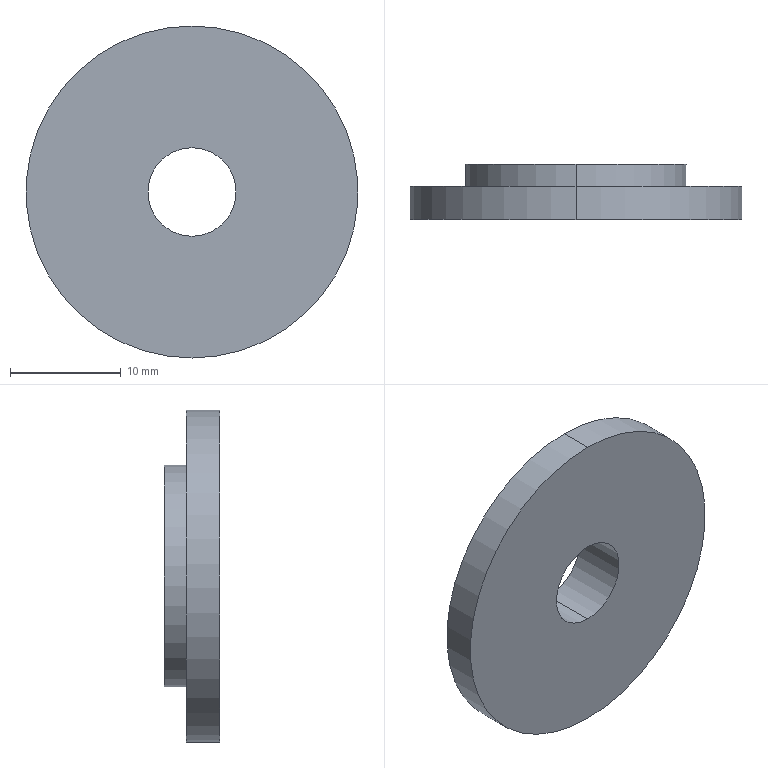Part | SolidWorks | features ICE 2, Extrusion 1 | 1 solid | 9 faces | box 30 x 5 x 30 mm | volume 2498 mm3 | cylinder 6 | plane 3 | commonest cylinder face diameters 8 x2 20 x2 30 x2
STEP:
#1=CARTESIAN_POINT('',(0.,0.,-4.));
#2=VERTEX_POINT('',#1);
#3=CARTESIAN_POINT('',(0.,0.,4.));
#4=VERTEX_POINT('',#3);
#5=CARTESIAN_POINT('',(0.,0.,0.));
#6=DIRECTION('',(0.,1.,0.));
#7=DIRECTION('',(0.,0.,1.));
#8=AXIS2_PLACEMENT_3D('',#5,#6,#7);
#9=CIRCLE('',#8,4.);
#10=EDGE_CURVE('',#2,#4,#9,.T.);
#11=ORIENTED_EDGE('',*,*,#10,.F.);
#12=CARTESIAN_POINT('',(0.,5.,-4.));
#13=VERTEX_POINT('',#12);
#14=CARTESIAN_POINT('',(0.,0.,-4.));
#15=DIRECTION('',(0.,1.,0.));
#16=VECTOR('',#15,1000.);
#17=LINE('',#14,#16);
#18=EDGE_CURVE('',#2,#13,#17,.T.);
#19=ORIENTED_EDGE('',*,*,#18,.T.);
#20=CARTESIAN_POINT('',(0.,5.,4.));
#21=VERTEX_POINT('',#20);
#22=CARTESIAN_POINT('',(0.,5.,0.));
#23=DIRECTION('',(0.,1.,0.));
#24=DIRECTION('',(0.,0.,1.));
#25=AXIS2_PLACEMENT_3D('',#22,#23,#24);
#26=CIRCLE('',#25,4.);
#27=EDGE_CURVE('',#13,#21,#26,.T.);
#28=ORIENTED_EDGE('',*,*,#27,.T.);
#29=CARTESIAN_POINT('',(0.,0.,4.));
#30=DIRECTION('',(0.,1.,0.));
#31=VECTOR('',#30,1000.);
#32=LINE('',#29,#31);
#33=EDGE_CURVE('',#4,#21,#32,.T.);
#34=ORIENTED_EDGE('',*,*,#33,.F.);
#35=EDGE_LOOP('',(#11,#19,#28,#34));
#36=FACE_OUTER_BOUND('',#35,.T.);
#37=CARTESIAN_POINT('',(0.,0.,0.));
#38=DIRECTION('',(0.,1.,0.));
#39=DIRECTION('',(0.,0.,1.));
#40=AXIS2_PLACEMENT_3D('',#37,#38,#39);
#41=CYLINDRICAL_SURFACE('',#40,4.);
#42=ADVANCED_FACE('',(#36),#41,.F.);
#43=CARTESIAN_POINT('',(0.,5.,10.));
#44=VERTEX_POINT('',#43);
#45=CARTESIAN_POINT('',(0.,5.,-10.));
#46=VERTEX_POINT('',#45);
#47=CARTESIAN_POINT('',(0.,5.,0.));
#48=DIRECTION('',(0.,1.,0.));
#49=DIRECTION('',(0.,0.,1.));
#50=AXIS2_PLACEMENT_3D('',#47,#48,#49);
#51=CIRCLE('',#50,10.);
#52=EDGE_CURVE('',#44,#46,#51,.T.);
#53=ORIENTED_EDGE('',*,*,#52,.F.);
#54=CARTESIAN_POINT('',(0.,3.,10.));
#55=VERTEX_POINT('',#54);
#56=CARTESIAN_POINT('',(0.,5.,10.));
#57=DIRECTION('',(0.,-1.,0.));
#58=VECTOR('',#57,1000.);
#59=LINE('',#56,#58);
#60=EDGE_CURVE('',#44,#55,#59,.T.);
#61=ORIENTED_EDGE('',*,*,#60,.T.);
#62=CARTESIAN_POINT('',(0.,3.,-10.));
#63=VERTEX_POINT('',#62);
#64=CARTESIAN_POINT('',(0.,3.,0.));
#65=DIRECTION('',(0.,1.,0.));
#66=DIRECTION('',(0.,0.,1.));
#67=AXIS2_PLACEMENT_3D('',#64,#65,#66);
#68=CIRCLE('',#67,10.);
#69=EDGE_CURVE('',#55,#63,#68,.T.);
#70=ORIENTED_EDGE('',*,*,#69,.T.);
#71=CARTESIAN_POINT('',(0.,5.,-10.));
#72=DIRECTION('',(0.,-1.,0.));
#73=VECTOR('',#72,1000.);
#74=LINE('',#71,#73);
#75=EDGE_CURVE('',#46,#63,#74,.T.);
#76=ORIENTED_EDGE('',*,*,#75,.F.);
#77=EDGE_LOOP('',(#53,#61,#70,#76));
#78=FACE_OUTER_BOUND('',#77,.T.);
#79=CARTESIAN_POINT('',(0.,5.,0.));
#80=DIRECTION('',(0.,-1.,0.));
#81=DIRECTION('',(0.,0.,-1.));
#82=AXIS2_PLACEMENT_3D('',#79,#80,#81);
#83=CYLINDRICAL_SURFACE('',#82,10.);
#84=ADVANCED_FACE('',(#78),#83,.T.);
#85=CARTESIAN_POINT('',(0.,3.,15.));
#86=VERTEX_POINT('',#85);
#87=CARTESIAN_POINT('',(0.,3.,-15.));
#88=VERTEX_POINT('',#87);
#89=CARTESIAN_POINT('',(0.,3.,0.));
#90=DIRECTION('',(0.,1.,0.));
#91=DIRECTION('',(0.,0.,1.));
#92=AXIS2_PLACEMENT_3D('',#89,#90,#91);
#93=CIRCLE('',#92,15.);
#94=EDGE_CURVE('',#86,#88,#93,.T.);
#95=ORIENTED_EDGE('',*,*,#94,.F.);
#96=CARTESIAN_POINT('',(0.,0.,15.));
#97=VERTEX_POINT('',#96);
#98=CARTESIAN_POINT('',(0.,3.,15.));
#99=DIRECTION('',(0.,-1.,0.));
#100=VECTOR('',#99,1000.);
#101=LINE('',#98,#100);
#102=EDGE_CURVE('',#86,#97,#101,.T.);
#103=ORIENTED_EDGE('',*,*,#102,.T.);
#104=CARTESIAN_POINT('',(0.,0.,-15.));
#105=VERTEX_POINT('',#104);
#106=CARTESIAN_POINT('',(0.,0.,0.));
#107=DIRECTION('',(0.,1.,0.));
#108=DIRECTION('',(0.,0.,1.));
#109=AXIS2_PLACEMENT_3D('',#106,#107,#108);
#110=CIRCLE('',#109,15.);
#111=EDGE_CURVE('',#97,#105,#110,.T.);
#112=ORIENTED_EDGE('',*,*,#111,.T.);
#113=CARTESIAN_POINT('',(0.,3.,-15.));
#114=DIRECTION('',(0.,-1.,0.));
#115=VECTOR('',#114,1000.);
#116=LINE('',#113,#115);
#117=EDGE_CURVE('',#88,#105,#116,.T.);
#118=ORIENTED_EDGE('',*,*,#117,.F.);
#119=EDGE_LOOP('',(#95,#103,#112,#118));
#120=FACE_OUTER_BOUND('',#119,.T.);
#121=CARTESIAN_POINT('',(0.,3.,0.));
#122=DIRECTION('',(0.,-1.,0.));
#123=DIRECTION('',(0.,0.,-1.));
#124=AXIS2_PLACEMENT_3D('',#121,#122,#123);
#125=CYLINDRICAL_SURFACE('',#124,15.);
#126=ADVANCED_FACE('',(#120),#125,.T.);
#127=CARTESIAN_POINT('',(0.,3.,0.));
#128=DIRECTION('',(0.,1.,0.));
#129=DIRECTION('',(0.,0.,1.));
#130=AXIS2_PLACEMENT_3D('',#127,#128,#129);
#131=CIRCLE('',#130,15.);
#132=EDGE_CURVE('',#88,#86,#131,.T.);
#133=ORIENTED_EDGE('',*,*,#132,.T.);
#134=ORIENTED_EDGE('',*,*,#94,.T.);
#135=EDGE_LOOP('',(#133,#134));
#136=FACE_OUTER_BOUND('',#135,.T.);
#137=CARTESIAN_POINT('',(0.,3.,0.));
#138=DIRECTION('',(0.,1.,0.));
#139=DIRECTION('',(0.,0.,1.));
#140=AXIS2_PLACEMENT_3D('',#137,#138,#139);
#141=CIRCLE('',#140,10.);
#142=EDGE_CURVE('',#63,#55,#141,.T.);
#143=ORIENTED_EDGE('',*,*,#142,.F.);
#144=ORIENTED_EDGE('',*,*,#69,.F.);
#145=EDGE_LOOP('',(#143,#144));
#146=FACE_BOUND('',#145,.T.);
#147=CARTESIAN_POINT('',(0.,3.,0.));
#148=DIRECTION('',(0.,1.,0.));
#149=DIRECTION('',(0.,0.,1.));
#150=AXIS2_PLACEMENT_3D('',#147,#148,#149);
#151=PLANE('',#150);
#152=ADVANCED_FACE('',(#136,#146),#151,.T.);
#153=ORIENTED_EDGE('',*,*,#102,.F.);
#154=ORIENTED_EDGE('',*,*,#132,.F.);
#155=ORIENTED_EDGE('',*,*,#117,.T.);
#156=CARTESIAN_POINT('',(0.,0.,0.));
#157=DIRECTION('',(0.,1.,0.));
#158=DIRECTION('',(0.,0.,1.));
#159=AXIS2_PLACEMENT_3D('',#156,#157,#158);
#160=CIRCLE('',#159,15.);
#161=EDGE_CURVE('',#105,#97,#160,.T.);
#162=ORIENTED_EDGE('',*,*,#161,.T.);
#163=EDGE_LOOP('',(#153,#154,#155,#162));
#164=FACE_OUTER_BOUND('',#163,.T.);
#165=CARTESIAN_POINT('',(0.,3.,0.));
#166=DIRECTION('',(0.,-1.,0.));
#167=DIRECTION('',(0.,0.,-1.));
#168=AXIS2_PLACEMENT_3D('',#165,#166,#167);
#169=CYLINDRICAL_SURFACE('',#168,15.);
#170=ADVANCED_FACE('',(#164),#169,.T.);
#171=CARTESIAN_POINT('',(0.,0.,0.));
#172=DIRECTION('',(0.,1.,0.));
#173=DIRECTION('',(0.,0.,1.));
#174=AXIS2_PLACEMENT_3D('',#171,#172,#173);
#175=CIRCLE('',#174,4.);
#176=EDGE_CURVE('',#4,#2,#175,.T.);
#177=ORIENTED_EDGE('',*,*,#176,.T.);
#178=ORIENTED_EDGE('',*,*,#10,.T.);
#179=EDGE_LOOP('',(#177,#178));
#180=FACE_BOUND('',#179,.T.);
#181=ORIENTED_EDGE('',*,*,#161,.F.);
#182=ORIENTED_EDGE('',*,*,#111,.F.);
#183=EDGE_LOOP('',(#181,#182));
#184=FACE_OUTER_BOUND('',#183,.T.);
#185=CARTESIAN_POINT('',(0.,0.,0.));
#186=DIRECTION('',(0.,1.,0.));
#187=DIRECTION('',(0.,0.,1.));
#188=AXIS2_PLACEMENT_3D('',#185,#186,#187);
#189=PLANE('',#188);
#190=ADVANCED_FACE('',(#180,#184),#189,.F.);
#191=ORIENTED_EDGE('',*,*,#60,.F.);
#192=CARTESIAN_POINT('',(0.,5.,0.));
#193=DIRECTION('',(0.,1.,0.));
#194=DIRECTION('',(0.,0.,1.));
#195=AXIS2_PLACEMENT_3D('',#192,#193,#194);
#196=CIRCLE('',#195,10.);
#197=EDGE_CURVE('',#46,#44,#196,.T.);
#198=ORIENTED_EDGE('',*,*,#197,.F.);
#199=ORIENTED_EDGE('',*,*,#75,.T.);
#200=ORIENTED_EDGE('',*,*,#142,.T.);
#201=EDGE_LOOP('',(#191,#198,#199,#200));
#202=FACE_OUTER_BOUND('',#201,.T.);
#203=CARTESIAN_POINT('',(0.,5.,0.));
#204=DIRECTION('',(0.,-1.,0.));
#205=DIRECTION('',(0.,0.,-1.));
#206=AXIS2_PLACEMENT_3D('',#203,#204,#205);
#207=CYLINDRICAL_SURFACE('',#206,10.);
#208=ADVANCED_FACE('',(#202),#207,.T.);
#209=CARTESIAN_POINT('',(0.,5.,0.));
#210=DIRECTION('',(0.,1.,0.));
#211=DIRECTION('',(0.,0.,1.));
#212=AXIS2_PLACEMENT_3D('',#209,#210,#211);
#213=CIRCLE('',#212,4.);
#214=EDGE_CURVE('',#21,#13,#213,.T.);
#215=ORIENTED_EDGE('',*,*,#214,.F.);
#216=ORIENTED_EDGE('',*,*,#27,.F.);
#217=EDGE_LOOP('',(#215,#216));
#218=FACE_BOUND('',#217,.T.);
#219=ORIENTED_EDGE('',*,*,#197,.T.);
#220=ORIENTED_EDGE('',*,*,#52,.T.);
#221=EDGE_LOOP('',(#219,#220));
#222=FACE_OUTER_BOUND('',#221,.T.);
#223=CARTESIAN_POINT('',(0.,5.,0.));
#224=DIRECTION('',(0.,1.,0.));
#225=DIRECTION('',(0.,0.,1.));
#226=AXIS2_PLACEMENT_3D('',#223,#224,#225);
#227=PLANE('',#226);
#228=ADVANCED_FACE('',(#218,#222),#227,.T.);
#229=ORIENTED_EDGE('',*,*,#18,.F.);
#230=ORIENTED_EDGE('',*,*,#176,.F.);
#231=ORIENTED_EDGE('',*,*,#33,.T.);
#232=ORIENTED_EDGE('',*,*,#214,.T.);
#233=EDGE_LOOP('',(#229,#230,#231,#232));
#234=FACE_OUTER_BOUND('',#233,.T.);
#235=CARTESIAN_POINT('',(0.,0.,0.));
#236=DIRECTION('',(0.,1.,0.));
#237=DIRECTION('',(0.,0.,1.));
#238=AXIS2_PLACEMENT_3D('',#235,#236,#237);
#239=CYLINDRICAL_SURFACE('',#238,4.);
#240=ADVANCED_FACE('',(#234),#239,.F.);
#241=CLOSED_SHELL('',(#42,#84,#126,#152,#170,#190,#208,#228,#240));
#242=MANIFOLD_SOLID_BREP('',#241);
#243=CARTESIAN_POINT('',(0.,0.,0.));
#244=DIRECTION('',(0.,0.,1.));
#245=DIRECTION('',(1.,0.,0.));
#246=AXIS2_PLACEMENT_3D('',#243,#244,#245);
#247=(LENGTH_UNIT()NAMED_UNIT(*)SI_UNIT(.MILLI.,.METRE.));
#248=UNCERTAINTY_MEASURE_WITH_UNIT(LENGTH_MEASURE(0.00001),#247,'','');
#249=(NAMED_UNIT(*)PLANE_ANGLE_UNIT()SI_UNIT($,.RADIAN.));
#250=(NAMED_UNIT(*)SI_UNIT($,.STERADIAN.)SOLID_ANGLE_UNIT());
#251=(GEOMETRIC_REPRESENTATION_CONTEXT(3)GLOBAL_UNCERTAINTY_ASSIGNED_CONTEXT((#248))GLOBAL_UNIT_ASSIGNED_CONTEXT((#247,#249,#250))REPRESENTATION_CONTEXT('',''));
#252=ADVANCED_BREP_SHAPE_REPRESENTATION('',(#242,#246),#251);